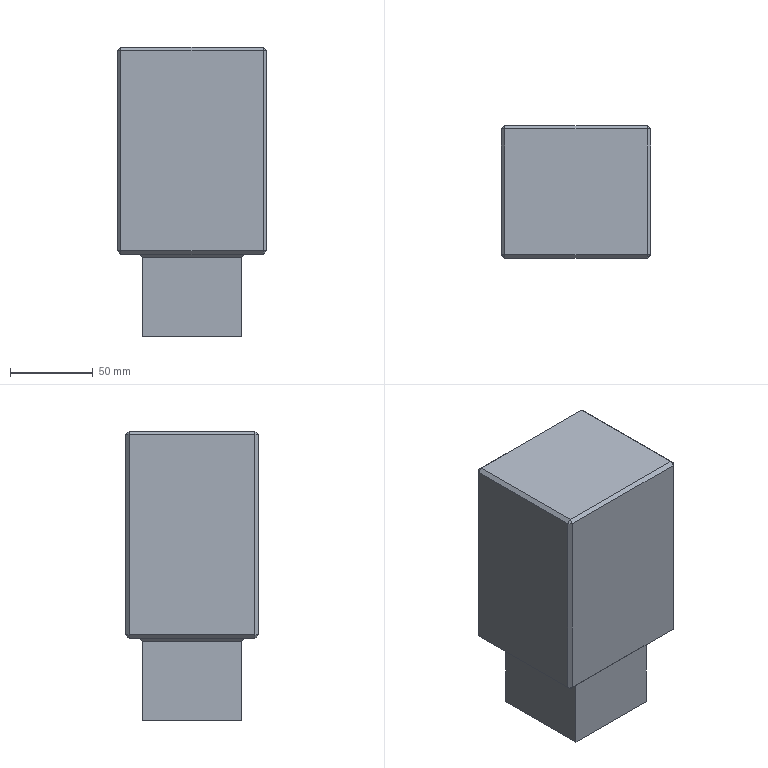Part | SolidWorks | features Boss 1, Chamfer 1, Cut 1, Extrusion 1 | 1 solid | 38 faces | box 90 x 80 x 175 mm | volume 1069126 mm3 | plane 36 | cylinder 2 | commonest cylinder face diameters 12 x2
STEP:
#1=CARTESIAN_POINT('',(36.,30.,80.));
#2=VERTEX_POINT('',#1);
#3=CARTESIAN_POINT('',(24.,30.,80.));
#4=VERTEX_POINT('',#3);
#5=CARTESIAN_POINT('',(30.,30.,80.));
#6=DIRECTION('',(0.,0.,-1.));
#7=DIRECTION('',(-1.,0.,0.));
#8=AXIS2_PLACEMENT_3D('',#5,#6,#7);
#9=CIRCLE('',#8,6.);
#10=EDGE_CURVE('',#2,#4,#9,.T.);
#11=ORIENTED_EDGE('',*,*,#10,.F.);
#12=CARTESIAN_POINT('',(36.,30.,0.));
#13=VERTEX_POINT('',#12);
#14=CARTESIAN_POINT('',(36.,30.,80.));
#15=DIRECTION('',(0.,0.,-1.));
#16=VECTOR('',#15,1000.);
#17=LINE('',#14,#16);
#18=EDGE_CURVE('',#2,#13,#17,.T.);
#19=ORIENTED_EDGE('',*,*,#18,.T.);
#20=CARTESIAN_POINT('',(24.,30.,0.));
#21=VERTEX_POINT('',#20);
#22=CARTESIAN_POINT('',(30.,30.,0.));
#23=DIRECTION('',(0.,0.,-1.));
#24=DIRECTION('',(-1.,0.,0.));
#25=AXIS2_PLACEMENT_3D('',#22,#23,#24);
#26=CIRCLE('',#25,6.);
#27=EDGE_CURVE('',#13,#21,#26,.T.);
#28=ORIENTED_EDGE('',*,*,#27,.T.);
#29=CARTESIAN_POINT('',(24.,30.,80.));
#30=DIRECTION('',(0.,0.,-1.));
#31=VECTOR('',#30,1000.);
#32=LINE('',#29,#31);
#33=EDGE_CURVE('',#4,#21,#32,.T.);
#34=ORIENTED_EDGE('',*,*,#33,.F.);
#35=EDGE_LOOP('',(#11,#19,#28,#34));
#36=FACE_OUTER_BOUND('',#35,.T.);
#37=CARTESIAN_POINT('',(30.,30.,80.));
#38=DIRECTION('',(0.,0.,-1.));
#39=DIRECTION('',(-1.,0.,0.));
#40=AXIS2_PLACEMENT_3D('',#37,#38,#39);
#41=CYLINDRICAL_SURFACE('',#40,6.);
#42=ADVANCED_FACE('',(#36),#41,.F.);
#43=CARTESIAN_POINT('',(0.,0.,48.));
#44=VERTEX_POINT('',#43);
#45=CARTESIAN_POINT('',(0.,0.,0.));
#46=VERTEX_POINT('',#45);
#47=CARTESIAN_POINT('',(0.,0.,50.));
#48=DIRECTION('',(0.,0.,-1.));
#49=VECTOR('',#48,1000.);
#50=LINE('',#47,#49);
#51=EDGE_CURVE('',#44,#46,#50,.T.);
#52=ORIENTED_EDGE('',*,*,#51,.F.);
#53=CARTESIAN_POINT('',(0.,60.,48.));
#54=VERTEX_POINT('',#53);
#55=CARTESIAN_POINT('',(0.,60.,48.));
#56=DIRECTION('',(0.,1.,0.));
#57=VECTOR('',#56,1000.);
#58=LINE('',#55,#57);
#59=EDGE_CURVE('',#44,#54,#58,.T.);
#60=ORIENTED_EDGE('',*,*,#59,.T.);
#61=CARTESIAN_POINT('',(0.,60.,0.));
#62=VERTEX_POINT('',#61);
#63=CARTESIAN_POINT('',(0.,60.,50.));
#64=DIRECTION('',(0.,0.,-1.));
#65=VECTOR('',#64,1000.);
#66=LINE('',#63,#65);
#67=EDGE_CURVE('',#54,#62,#66,.T.);
#68=ORIENTED_EDGE('',*,*,#67,.T.);
#69=CARTESIAN_POINT('',(0.,0.,0.));
#70=DIRECTION('',(0.,-1.,0.));
#71=VECTOR('',#70,1000.);
#72=LINE('',#69,#71);
#73=EDGE_CURVE('',#62,#46,#72,.T.);
#74=ORIENTED_EDGE('',*,*,#73,.T.);
#75=EDGE_LOOP('',(#52,#60,#68,#74));
#76=FACE_OUTER_BOUND('',#75,.T.);
#77=CARTESIAN_POINT('',(0.,0.,50.));
#78=DIRECTION('',(1.,0.,0.));
#79=DIRECTION('',(0.,0.,-1.));
#80=AXIS2_PLACEMENT_3D('',#77,#78,#79);
#81=PLANE('',#80);
#82=ADVANCED_FACE('',(#76),#81,.F.);
#83=CARTESIAN_POINT('',(60.,0.,48.));
#84=VERTEX_POINT('',#83);
#85=CARTESIAN_POINT('',(60.,0.,0.));
#86=VERTEX_POINT('',#85);
#87=CARTESIAN_POINT('',(60.,0.,50.));
#88=DIRECTION('',(0.,0.,-1.));
#89=VECTOR('',#88,1000.);
#90=LINE('',#87,#89);
#91=EDGE_CURVE('',#84,#86,#90,.T.);
#92=ORIENTED_EDGE('',*,*,#91,.F.);
#93=CARTESIAN_POINT('',(0.,0.,48.));
#94=DIRECTION('',(-1.,0.,0.));
#95=VECTOR('',#94,1000.);
#96=LINE('',#93,#95);
#97=EDGE_CURVE('',#84,#44,#96,.T.);
#98=ORIENTED_EDGE('',*,*,#97,.T.);
#99=ORIENTED_EDGE('',*,*,#51,.T.);
#100=CARTESIAN_POINT('',(0.,0.,0.));
#101=DIRECTION('',(1.,0.,0.));
#102=VECTOR('',#101,1000.);
#103=LINE('',#100,#102);
#104=EDGE_CURVE('',#46,#86,#103,.T.);
#105=ORIENTED_EDGE('',*,*,#104,.T.);
#106=EDGE_LOOP('',(#92,#98,#99,#105));
#107=FACE_OUTER_BOUND('',#106,.T.);
#108=CARTESIAN_POINT('',(0.,0.,50.));
#109=DIRECTION('',(0.,1.,0.));
#110=DIRECTION('',(0.,0.,1.));
#111=AXIS2_PLACEMENT_3D('',#108,#109,#110);
#112=PLANE('',#111);
#113=ADVANCED_FACE('',(#107),#112,.F.);
#114=CARTESIAN_POINT('',(60.,60.,48.));
#115=VERTEX_POINT('',#114);
#116=CARTESIAN_POINT('',(60.,60.,0.));
#117=VERTEX_POINT('',#116);
#118=CARTESIAN_POINT('',(60.,60.,50.));
#119=DIRECTION('',(0.,0.,-1.));
#120=VECTOR('',#119,1000.);
#121=LINE('',#118,#120);
#122=EDGE_CURVE('',#115,#117,#121,.T.);
#123=ORIENTED_EDGE('',*,*,#122,.F.);
#124=CARTESIAN_POINT('',(60.,0.,48.));
#125=DIRECTION('',(0.,-1.,0.));
#126=VECTOR('',#125,1000.);
#127=LINE('',#124,#126);
#128=EDGE_CURVE('',#115,#84,#127,.T.);
#129=ORIENTED_EDGE('',*,*,#128,.T.);
#130=ORIENTED_EDGE('',*,*,#91,.T.);
#131=CARTESIAN_POINT('',(60.,0.,0.));
#132=DIRECTION('',(0.,1.,0.));
#133=VECTOR('',#132,1000.);
#134=LINE('',#131,#133);
#135=EDGE_CURVE('',#86,#117,#134,.T.);
#136=ORIENTED_EDGE('',*,*,#135,.T.);
#137=EDGE_LOOP('',(#123,#129,#130,#136));
#138=FACE_OUTER_BOUND('',#137,.T.);
#139=CARTESIAN_POINT('',(60.,0.,50.));
#140=DIRECTION('',(-1.,0.,0.));
#141=DIRECTION('',(0.,0.,1.));
#142=AXIS2_PLACEMENT_3D('',#139,#140,#141);
#143=PLANE('',#142);
#144=ADVANCED_FACE('',(#138),#143,.F.);
#145=ORIENTED_EDGE('',*,*,#67,.F.);
#146=CARTESIAN_POINT('',(60.,60.,48.));
#147=DIRECTION('',(1.,0.,0.));
#148=VECTOR('',#147,1000.);
#149=LINE('',#146,#148);
#150=EDGE_CURVE('',#54,#115,#149,.T.);
#151=ORIENTED_EDGE('',*,*,#150,.T.);
#152=ORIENTED_EDGE('',*,*,#122,.T.);
#153=CARTESIAN_POINT('',(0.,60.,0.));
#154=DIRECTION('',(-1.,0.,0.));
#155=VECTOR('',#154,1000.);
#156=LINE('',#153,#155);
#157=EDGE_CURVE('',#117,#62,#156,.T.);
#158=ORIENTED_EDGE('',*,*,#157,.T.);
#159=EDGE_LOOP('',(#145,#151,#152,#158));
#160=FACE_OUTER_BOUND('',#159,.T.);
#161=CARTESIAN_POINT('',(0.,60.,50.));
#162=DIRECTION('',(0.,-1.,0.));
#163=DIRECTION('',(0.,0.,-1.));
#164=AXIS2_PLACEMENT_3D('',#161,#162,#163);
#165=PLANE('',#164);
#166=ADVANCED_FACE('',(#160),#165,.F.);
#167=CARTESIAN_POINT('',(30.,30.,0.));
#168=DIRECTION('',(0.,0.,-1.));
#169=DIRECTION('',(-1.,0.,0.));
#170=AXIS2_PLACEMENT_3D('',#167,#168,#169);
#171=CIRCLE('',#170,6.);
#172=EDGE_CURVE('',#21,#13,#171,.T.);
#173=ORIENTED_EDGE('',*,*,#172,.F.);
#174=ORIENTED_EDGE('',*,*,#27,.F.);
#175=EDGE_LOOP('',(#173,#174));
#176=FACE_BOUND('',#175,.T.);
#177=ORIENTED_EDGE('',*,*,#73,.F.);
#178=ORIENTED_EDGE('',*,*,#157,.F.);
#179=ORIENTED_EDGE('',*,*,#135,.F.);
#180=ORIENTED_EDGE('',*,*,#104,.F.);
#181=EDGE_LOOP('',(#177,#178,#179,#180));
#182=FACE_OUTER_BOUND('',#181,.T.);
#183=CARTESIAN_POINT('',(0.,60.,0.));
#184=DIRECTION('',(0.,0.,-1.));
#185=DIRECTION('',(-1.,0.,0.));
#186=AXIS2_PLACEMENT_3D('',#183,#184,#185);
#187=PLANE('',#186);
#188=ADVANCED_FACE('',(#176,#182),#187,.T.);
#189=CARTESIAN_POINT('',(-2.,-2.,50.));
#190=VERTEX_POINT('',#189);
#191=CARTESIAN_POINT('',(62.,-2.,50.));
#192=VERTEX_POINT('',#191);
#193=CARTESIAN_POINT('',(60.,-2.,50.));
#194=DIRECTION('',(1.,0.,0.));
#195=VECTOR('',#194,1000.);
#196=LINE('',#193,#195);
#197=EDGE_CURVE('',#190,#192,#196,.T.);
#198=ORIENTED_EDGE('',*,*,#197,.T.);
#199=CARTESIAN_POINT('',(62.,62.,50.));
#200=VERTEX_POINT('',#199);
#201=CARTESIAN_POINT('',(62.,60.,50.));
#202=DIRECTION('',(0.,1.,0.));
#203=VECTOR('',#202,1000.);
#204=LINE('',#201,#203);
#205=EDGE_CURVE('',#192,#200,#204,.T.);
#206=ORIENTED_EDGE('',*,*,#205,.T.);
#207=CARTESIAN_POINT('',(-2.,62.,50.));
#208=VERTEX_POINT('',#207);
#209=CARTESIAN_POINT('',(0.,62.,50.));
#210=DIRECTION('',(-1.,0.,0.));
#211=VECTOR('',#210,1000.);
#212=LINE('',#209,#211);
#213=EDGE_CURVE('',#200,#208,#212,.T.);
#214=ORIENTED_EDGE('',*,*,#213,.T.);
#215=CARTESIAN_POINT('',(-2.,0.,50.));
#216=DIRECTION('',(0.,-1.,0.));
#217=VECTOR('',#216,1000.);
#218=LINE('',#215,#217);
#219=EDGE_CURVE('',#208,#190,#218,.T.);
#220=ORIENTED_EDGE('',*,*,#219,.T.);
#221=EDGE_LOOP('',(#198,#206,#214,#220));
#222=FACE_BOUND('',#221,.T.);
#223=CARTESIAN_POINT('',(73.,68.,50.));
#224=VERTEX_POINT('',#223);
#225=CARTESIAN_POINT('',(73.,-8.,50.));
#226=VERTEX_POINT('',#225);
#227=CARTESIAN_POINT('',(73.,-10.,50.));
#228=DIRECTION('',(0.,-1.,0.));
#229=VECTOR('',#228,1000.);
#230=LINE('',#227,#229);
#231=EDGE_CURVE('',#224,#226,#230,.T.);
#232=ORIENTED_EDGE('',*,*,#231,.T.);
#233=CARTESIAN_POINT('',(-13.,-8.,50.));
#234=VERTEX_POINT('',#233);
#235=CARTESIAN_POINT('',(-15.,-8.,50.));
#236=DIRECTION('',(-1.,0.,0.));
#237=VECTOR('',#236,1000.);
#238=LINE('',#235,#237);
#239=EDGE_CURVE('',#226,#234,#238,.T.);
#240=ORIENTED_EDGE('',*,*,#239,.T.);
#241=CARTESIAN_POINT('',(-13.,68.,50.));
#242=VERTEX_POINT('',#241);
#243=CARTESIAN_POINT('',(-13.,-10.,50.));
#244=DIRECTION('',(0.,1.,0.));
#245=VECTOR('',#244,1000.);
#246=LINE('',#243,#245);
#247=EDGE_CURVE('',#234,#242,#246,.T.);
#248=ORIENTED_EDGE('',*,*,#247,.T.);
#249=CARTESIAN_POINT('',(-15.,68.,50.));
#250=DIRECTION('',(1.,0.,0.));
#251=VECTOR('',#250,1000.);
#252=LINE('',#249,#251);
#253=EDGE_CURVE('',#242,#224,#252,.T.);
#254=ORIENTED_EDGE('',*,*,#253,.T.);
#255=EDGE_LOOP('',(#232,#240,#248,#254));
#256=FACE_OUTER_BOUND('',#255,.T.);
#257=CARTESIAN_POINT('',(-15.,-10.,50.));
#258=DIRECTION('',(0.,0.,1.));
#259=DIRECTION('',(1.,0.,0.));
#260=AXIS2_PLACEMENT_3D('',#257,#258,#259);
#261=PLANE('',#260);
#262=ADVANCED_FACE('',(#222,#256),#261,.F.);
#263=CARTESIAN_POINT('',(-15.,-8.,173.));
#264=VERTEX_POINT('',#263);
#265=CARTESIAN_POINT('',(-15.,68.,173.));
#266=VERTEX_POINT('',#265);
#267=CARTESIAN_POINT('',(-15.,70.,173.));
#268=DIRECTION('',(0.,1.,0.));
#269=VECTOR('',#268,1000.);
#270=LINE('',#267,#269);
#271=EDGE_CURVE('',#264,#266,#270,.T.);
#272=ORIENTED_EDGE('',*,*,#271,.T.);
#273=CARTESIAN_POINT('',(-15.,68.,52.));
#274=VERTEX_POINT('',#273);
#275=CARTESIAN_POINT('',(-15.,68.,175.));
#276=DIRECTION('',(0.,0.,-1.));
#277=VECTOR('',#276,1000.);
#278=LINE('',#275,#277);
#279=EDGE_CURVE('',#266,#274,#278,.T.);
#280=ORIENTED_EDGE('',*,*,#279,.T.);
#281=CARTESIAN_POINT('',(-15.,-8.,52.));
#282=VERTEX_POINT('',#281);
#283=CARTESIAN_POINT('',(-15.,70.,52.));
#284=DIRECTION('',(0.,-1.,0.));
#285=VECTOR('',#284,1000.);
#286=LINE('',#283,#285);
#287=EDGE_CURVE('',#274,#282,#286,.T.);
#288=ORIENTED_EDGE('',*,*,#287,.T.);
#289=CARTESIAN_POINT('',(-15.,-8.,175.));
#290=DIRECTION('',(0.,0.,1.));
#291=VECTOR('',#290,1000.);
#292=LINE('',#289,#291);
#293=EDGE_CURVE('',#282,#264,#292,.T.);
#294=ORIENTED_EDGE('',*,*,#293,.T.);
#295=EDGE_LOOP('',(#272,#280,#288,#294));
#296=FACE_OUTER_BOUND('',#295,.T.);
#297=CARTESIAN_POINT('',(-15.,70.,175.));
#298=DIRECTION('',(1.,0.,0.));
#299=DIRECTION('',(0.,1.,0.));
#300=AXIS2_PLACEMENT_3D('',#297,#298,#299);
#301=PLANE('',#300);
#302=ADVANCED_FACE('',(#296),#301,.F.);
#303=CARTESIAN_POINT('',(73.,-10.,52.));
#304=VERTEX_POINT('',#303);
#305=CARTESIAN_POINT('',(73.,-10.,173.));
#306=VERTEX_POINT('',#305);
#307=CARTESIAN_POINT('',(73.,-10.,175.));
#308=DIRECTION('',(0.,0.,1.));
#309=VECTOR('',#308,1000.);
#310=LINE('',#307,#309);
#311=EDGE_CURVE('',#304,#306,#310,.T.);
#312=ORIENTED_EDGE('',*,*,#311,.T.);
#313=CARTESIAN_POINT('',(-13.,-10.,173.));
#314=VERTEX_POINT('',#313);
#315=CARTESIAN_POINT('',(-15.,-10.,173.));
#316=DIRECTION('',(-1.,0.,0.));
#317=VECTOR('',#316,1000.);
#318=LINE('',#315,#317);
#319=EDGE_CURVE('',#306,#314,#318,.T.);
#320=ORIENTED_EDGE('',*,*,#319,.T.);
#321=CARTESIAN_POINT('',(-13.,-10.,52.));
#322=VERTEX_POINT('',#321);
#323=CARTESIAN_POINT('',(-13.,-10.,175.));
#324=DIRECTION('',(0.,0.,-1.));
#325=VECTOR('',#324,1000.);
#326=LINE('',#323,#325);
#327=EDGE_CURVE('',#314,#322,#326,.T.);
#328=ORIENTED_EDGE('',*,*,#327,.T.);
#329=CARTESIAN_POINT('',(-15.,-10.,52.));
#330=DIRECTION('',(1.,0.,0.));
#331=VECTOR('',#330,1000.);
#332=LINE('',#329,#331);
#333=EDGE_CURVE('',#322,#304,#332,.T.);
#334=ORIENTED_EDGE('',*,*,#333,.T.);
#335=EDGE_LOOP('',(#312,#320,#328,#334));
#336=FACE_OUTER_BOUND('',#335,.T.);
#337=CARTESIAN_POINT('',(-15.,-10.,175.));
#338=DIRECTION('',(0.,1.,0.));
#339=DIRECTION('',(-1.,0.,0.));
#340=AXIS2_PLACEMENT_3D('',#337,#338,#339);
#341=PLANE('',#340);
#342=ADVANCED_FACE('',(#336),#341,.F.);
#343=CARTESIAN_POINT('',(75.,-8.,52.));
#344=VERTEX_POINT('',#343);
#345=CARTESIAN_POINT('',(75.,68.,52.));
#346=VERTEX_POINT('',#345);
#347=CARTESIAN_POINT('',(75.,70.,52.));
#348=DIRECTION('',(0.,1.,0.));
#349=VECTOR('',#348,1000.);
#350=LINE('',#347,#349);
#351=EDGE_CURVE('',#344,#346,#350,.T.);
#352=ORIENTED_EDGE('',*,*,#351,.T.);
#353=CARTESIAN_POINT('',(75.,68.,173.));
#354=VERTEX_POINT('',#353);
#355=CARTESIAN_POINT('',(75.,68.,175.));
#356=DIRECTION('',(0.,0.,1.));
#357=VECTOR('',#356,1000.);
#358=LINE('',#355,#357);
#359=EDGE_CURVE('',#346,#354,#358,.T.);
#360=ORIENTED_EDGE('',*,*,#359,.T.);
#361=CARTESIAN_POINT('',(75.,-8.,173.));
#362=VERTEX_POINT('',#361);
#363=CARTESIAN_POINT('',(75.,-10.,173.));
#364=DIRECTION('',(0.,-1.,0.));
#365=VECTOR('',#364,1000.);
#366=LINE('',#363,#365);
#367=EDGE_CURVE('',#354,#362,#366,.T.);
#368=ORIENTED_EDGE('',*,*,#367,.T.);
#369=CARTESIAN_POINT('',(75.,-8.,175.));
#370=DIRECTION('',(0.,0.,-1.));
#371=VECTOR('',#370,1000.);
#372=LINE('',#369,#371);
#373=EDGE_CURVE('',#362,#344,#372,.T.);
#374=ORIENTED_EDGE('',*,*,#373,.T.);
#375=EDGE_LOOP('',(#352,#360,#368,#374));
#376=FACE_OUTER_BOUND('',#375,.T.);
#377=CARTESIAN_POINT('',(75.,70.,175.));
#378=DIRECTION('',(-1.,0.,0.));
#379=DIRECTION('',(0.,-1.,0.));
#380=AXIS2_PLACEMENT_3D('',#377,#378,#379);
#381=PLANE('',#380);
#382=ADVANCED_FACE('',(#376),#381,.F.);
#383=CARTESIAN_POINT('',(-13.,70.,173.));
#384=VERTEX_POINT('',#383);
#385=CARTESIAN_POINT('',(73.,70.,173.));
#386=VERTEX_POINT('',#385);
#387=CARTESIAN_POINT('',(75.,70.,173.));
#388=DIRECTION('',(1.,0.,0.));
#389=VECTOR('',#388,1000.);
#390=LINE('',#387,#389);
#391=EDGE_CURVE('',#384,#386,#390,.T.);
#392=ORIENTED_EDGE('',*,*,#391,.T.);
#393=CARTESIAN_POINT('',(73.,70.,52.));
#394=VERTEX_POINT('',#393);
#395=CARTESIAN_POINT('',(73.,70.,175.));
#396=DIRECTION('',(0.,0.,-1.));
#397=VECTOR('',#396,1000.);
#398=LINE('',#395,#397);
#399=EDGE_CURVE('',#386,#394,#398,.T.);
#400=ORIENTED_EDGE('',*,*,#399,.T.);
#401=CARTESIAN_POINT('',(-13.,70.,52.));
#402=VERTEX_POINT('',#401);
#403=CARTESIAN_POINT('',(-15.,70.,52.));
#404=DIRECTION('',(-1.,0.,0.));
#405=VECTOR('',#404,1000.);
#406=LINE('',#403,#405);
#407=EDGE_CURVE('',#394,#402,#406,.T.);
#408=ORIENTED_EDGE('',*,*,#407,.T.);
#409=CARTESIAN_POINT('',(-13.,70.,175.));
#410=DIRECTION('',(0.,0.,1.));
#411=VECTOR('',#410,1000.);
#412=LINE('',#409,#411);
#413=EDGE_CURVE('',#402,#384,#412,.T.);
#414=ORIENTED_EDGE('',*,*,#413,.T.);
#415=EDGE_LOOP('',(#392,#400,#408,#414));
#416=FACE_OUTER_BOUND('',#415,.T.);
#417=CARTESIAN_POINT('',(-15.,70.,175.));
#418=DIRECTION('',(0.,-1.,0.));
#419=DIRECTION('',(0.,0.,-1.));
#420=AXIS2_PLACEMENT_3D('',#417,#418,#419);
#421=PLANE('',#420);
#422=ADVANCED_FACE('',(#416),#421,.F.);
#423=CARTESIAN_POINT('',(73.,-8.,175.));
#424=VERTEX_POINT('',#423);
#425=CARTESIAN_POINT('',(73.,68.,175.));
#426=VERTEX_POINT('',#425);
#427=CARTESIAN_POINT('',(73.,70.,175.));
#428=DIRECTION('',(0.,1.,0.));
#429=VECTOR('',#428,1000.);
#430=LINE('',#427,#429);
#431=EDGE_CURVE('',#424,#426,#430,.T.);
#432=ORIENTED_EDGE('',*,*,#431,.T.);
#433=CARTESIAN_POINT('',(-13.,68.,175.));
#434=VERTEX_POINT('',#433);
#435=CARTESIAN_POINT('',(-15.,68.,175.));
#436=DIRECTION('',(-1.,0.,0.));
#437=VECTOR('',#436,1000.);
#438=LINE('',#435,#437);
#439=EDGE_CURVE('',#426,#434,#438,.T.);
#440=ORIENTED_EDGE('',*,*,#439,.T.);
#441=CARTESIAN_POINT('',(-13.,-8.,175.));
#442=VERTEX_POINT('',#441);
#443=CARTESIAN_POINT('',(-13.,-10.,175.));
#444=DIRECTION('',(0.,-1.,0.));
#445=VECTOR('',#444,1000.);
#446=LINE('',#443,#445);
#447=EDGE_CURVE('',#434,#442,#446,.T.);
#448=ORIENTED_EDGE('',*,*,#447,.T.);
#449=CARTESIAN_POINT('',(75.,-8.,175.));
#450=DIRECTION('',(1.,0.,0.));
#451=VECTOR('',#450,1000.);
#452=LINE('',#449,#451);
#453=EDGE_CURVE('',#442,#424,#452,.T.);
#454=ORIENTED_EDGE('',*,*,#453,.T.);
#455=EDGE_LOOP('',(#432,#440,#448,#454));
#456=FACE_OUTER_BOUND('',#455,.T.);
#457=CARTESIAN_POINT('',(-15.,-10.,175.));
#458=DIRECTION('',(0.,0.,1.));
#459=DIRECTION('',(1.,0.,0.));
#460=AXIS2_PLACEMENT_3D('',#457,#458,#459);
#461=PLANE('',#460);
#462=ADVANCED_FACE('',(#456),#461,.T.);
#463=CARTESIAN_POINT('',(-6.333,66.333,54.333));
#464=DIRECTION('',(-0.5774,0.5774,0.5774));
#465=VECTOR('',#464,1000.);
#466=LINE('',#463,#465);
#467=EDGE_CURVE('',#54,#208,#466,.T.);
#468=ORIENTED_EDGE('',*,*,#467,.F.);
#469=ORIENTED_EDGE('',*,*,#59,.F.);
#470=CARTESIAN_POINT('',(-4.667,-4.667,52.667));
#471=DIRECTION('',(0.5774,0.5774,-0.5774));
#472=VECTOR('',#471,1000.);
#473=LINE('',#470,#472);
#474=EDGE_CURVE('',#190,#44,#473,.T.);
#475=ORIENTED_EDGE('',*,*,#474,.F.);
#476=ORIENTED_EDGE('',*,*,#219,.F.);
#477=EDGE_LOOP('',(#468,#469,#475,#476));
#478=FACE_OUTER_BOUND('',#477,.T.);
#479=CARTESIAN_POINT('',(-2.,-10.,50.));
#480=DIRECTION('',(-0.7071,0.,-0.7071));
#481=DIRECTION('',(-0.7071,0.,0.7071));
#482=AXIS2_PLACEMENT_3D('',#479,#480,#481);
#483=PLANE('',#482);
#484=ADVANCED_FACE('',(#478),#483,.T.);
#485=ORIENTED_EDGE('',*,*,#474,.T.);
#486=ORIENTED_EDGE('',*,*,#97,.F.);
#487=CARTESIAN_POINT('',(36.333,23.667,24.333));
#488=DIRECTION('',(-0.5774,0.5774,-0.5774));
#489=VECTOR('',#488,1000.);
#490=LINE('',#487,#489);
#491=EDGE_CURVE('',#192,#84,#490,.T.);
#492=ORIENTED_EDGE('',*,*,#491,.F.);
#493=ORIENTED_EDGE('',*,*,#197,.F.);
#494=EDGE_LOOP('',(#485,#486,#492,#493));
#495=FACE_OUTER_BOUND('',#494,.T.);
#496=CARTESIAN_POINT('',(-15.,-2.,50.));
#497=DIRECTION('',(0.,-0.7071,-0.7071));
#498=DIRECTION('',(0.,0.7071,-0.7071));
#499=AXIS2_PLACEMENT_3D('',#496,#497,#498);
#500=PLANE('',#499);
#501=ADVANCED_FACE('',(#495),#500,.T.);
#502=ORIENTED_EDGE('',*,*,#467,.T.);
#503=ORIENTED_EDGE('',*,*,#213,.F.);
#504=CARTESIAN_POINT('',(36.333,36.333,24.333));
#505=DIRECTION('',(0.5774,0.5774,0.5774));
#506=VECTOR('',#505,1000.);
#507=LINE('',#504,#506);
#508=EDGE_CURVE('',#115,#200,#507,.T.);
#509=ORIENTED_EDGE('',*,*,#508,.F.);
#510=ORIENTED_EDGE('',*,*,#150,.F.);
#511=EDGE_LOOP('',(#502,#503,#509,#510));
#512=FACE_OUTER_BOUND('',#511,.T.);
#513=CARTESIAN_POINT('',(-15.,62.,50.));
#514=DIRECTION('',(0.,0.7071,-0.7071));
#515=DIRECTION('',(0.,0.7071,0.7071));
#516=AXIS2_PLACEMENT_3D('',#513,#514,#515);
#517=PLANE('',#516);
#518=ADVANCED_FACE('',(#512),#517,.T.);
#519=ORIENTED_EDGE('',*,*,#491,.T.);
#520=ORIENTED_EDGE('',*,*,#128,.F.);
#521=ORIENTED_EDGE('',*,*,#508,.T.);
#522=ORIENTED_EDGE('',*,*,#205,.F.);
#523=EDGE_LOOP('',(#519,#520,#521,#522));
#524=FACE_OUTER_BOUND('',#523,.T.);
#525=CARTESIAN_POINT('',(62.,-10.,50.));
#526=DIRECTION('',(0.7071,0.,-0.7071));
#527=DIRECTION('',(-0.7071,0.,-0.7071));
#528=AXIS2_PLACEMENT_3D('',#525,#526,#527);
#529=PLANE('',#528);
#530=ADVANCED_FACE('',(#524),#529,.T.);
#531=CARTESIAN_POINT('',(-13.,-10.,173.));
#532=DIRECTION('',(0.7071,-0.7071,0.));
#533=VECTOR('',#532,1000.);
#534=LINE('',#531,#533);
#535=EDGE_CURVE('',#264,#314,#534,.T.);
#536=ORIENTED_EDGE('',*,*,#535,.F.);
#537=ORIENTED_EDGE('',*,*,#293,.F.);
#538=CARTESIAN_POINT('',(-14.,-9.,52.));
#539=DIRECTION('',(-0.7071,0.7071,0.));
#540=VECTOR('',#539,1000.);
#541=LINE('',#538,#540);
#542=EDGE_CURVE('',#322,#282,#541,.T.);
#543=ORIENTED_EDGE('',*,*,#542,.F.);
#544=ORIENTED_EDGE('',*,*,#327,.F.);
#545=EDGE_LOOP('',(#536,#537,#543,#544));
#546=FACE_OUTER_BOUND('',#545,.T.);
#547=CARTESIAN_POINT('',(-13.,-10.,175.));
#548=DIRECTION('',(0.7071,0.7071,0.));
#549=DIRECTION('',(-0.7071,0.7071,0.));
#550=AXIS2_PLACEMENT_3D('',#547,#548,#549);
#551=PLANE('',#550);
#552=ADVANCED_FACE('',(#546),#551,.F.);
#553=CARTESIAN_POINT('',(-14.,-8.,174.));
#554=DIRECTION('',(0.7071,0.,0.7071));
#555=VECTOR('',#554,1000.);
#556=LINE('',#553,#555);
#557=EDGE_CURVE('',#264,#442,#556,.T.);
#558=ORIENTED_EDGE('',*,*,#557,.F.);
#559=ORIENTED_EDGE('',*,*,#535,.T.);
#560=CARTESIAN_POINT('',(-13.,-10.,173.));
#561=DIRECTION('',(0.,-0.7071,-0.7071));
#562=VECTOR('',#561,1000.);
#563=LINE('',#560,#562);
#564=EDGE_CURVE('',#442,#314,#563,.T.);
#565=ORIENTED_EDGE('',*,*,#564,.F.);
#566=EDGE_LOOP('',(#558,#559,#565));
#567=FACE_OUTER_BOUND('',#566,.T.);
#568=CARTESIAN_POINT('',(-13.,-10.,173.));
#569=DIRECTION('',(-0.5774,-0.5774,0.5774));
#570=DIRECTION('',(0.7071,-0.7071,0.));
#571=AXIS2_PLACEMENT_3D('',#568,#569,#570);
#572=PLANE('',#571);
#573=ADVANCED_FACE('',(#567),#572,.T.);
#574=CARTESIAN_POINT('',(-13.,-8.,50.));
#575=DIRECTION('',(0.,0.7071,-0.7071));
#576=VECTOR('',#575,1000.);
#577=LINE('',#574,#576);
#578=EDGE_CURVE('',#322,#234,#577,.T.);
#579=ORIENTED_EDGE('',*,*,#578,.F.);
#580=ORIENTED_EDGE('',*,*,#542,.T.);
#581=CARTESIAN_POINT('',(-13.,-8.,50.));
#582=DIRECTION('',(-0.7071,0.,0.7071));
#583=VECTOR('',#582,1000.);
#584=LINE('',#581,#583);
#585=EDGE_CURVE('',#234,#282,#584,.T.);
#586=ORIENTED_EDGE('',*,*,#585,.F.);
#587=EDGE_LOOP('',(#579,#580,#586));
#588=FACE_OUTER_BOUND('',#587,.T.);
#589=CARTESIAN_POINT('',(-13.,-8.,50.));
#590=DIRECTION('',(-0.5774,-0.5774,-0.5774));
#591=DIRECTION('',(-0.7071,0.,0.7071));
#592=AXIS2_PLACEMENT_3D('',#589,#590,#591);
#593=PLANE('',#592);
#594=ADVANCED_FACE('',(#588),#593,.T.);
#595=ORIENTED_EDGE('',*,*,#564,.T.);
#596=ORIENTED_EDGE('',*,*,#319,.F.);
#597=CARTESIAN_POINT('',(73.,-9.,174.));
#598=DIRECTION('',(0.,-0.7071,-0.7071));
#599=VECTOR('',#598,1000.);
#600=LINE('',#597,#599);
#601=EDGE_CURVE('',#424,#306,#600,.T.);
#602=ORIENTED_EDGE('',*,*,#601,.F.);
#603=ORIENTED_EDGE('',*,*,#453,.F.);
#604=EDGE_LOOP('',(#595,#596,#602,#603));
#605=FACE_OUTER_BOUND('',#604,.T.);
#606=CARTESIAN_POINT('',(-15.,-8.,175.));
#607=DIRECTION('',(0.,-0.7071,0.7071));
#608=DIRECTION('',(0.,-0.7071,-0.7071));
#609=AXIS2_PLACEMENT_3D('',#606,#607,#608);
#610=PLANE('',#609);
#611=ADVANCED_FACE('',(#605),#610,.T.);
#612=ORIENTED_EDGE('',*,*,#557,.T.);
#613=ORIENTED_EDGE('',*,*,#447,.F.);
#614=CARTESIAN_POINT('',(-13.,68.,175.));
#615=DIRECTION('',(0.7071,0.,0.7071));
#616=VECTOR('',#615,1000.);
#617=LINE('',#614,#616);
#618=EDGE_CURVE('',#266,#434,#617,.T.);
#619=ORIENTED_EDGE('',*,*,#618,.F.);
#620=ORIENTED_EDGE('',*,*,#271,.F.);
#621=EDGE_LOOP('',(#612,#613,#619,#620));
#622=FACE_OUTER_BOUND('',#621,.T.);
#623=CARTESIAN_POINT('',(-13.,-10.,175.));
#624=DIRECTION('',(-0.7071,0.,0.7071));
#625=DIRECTION('',(0.7071,0.,0.7071));
#626=AXIS2_PLACEMENT_3D('',#623,#624,#625);
#627=PLANE('',#626);
#628=ADVANCED_FACE('',(#622),#627,.T.);
#629=CARTESIAN_POINT('',(-13.,70.,52.));
#630=DIRECTION('',(0.7071,0.7071,0.));
#631=VECTOR('',#630,1000.);
#632=LINE('',#629,#631);
#633=EDGE_CURVE('',#274,#402,#632,.T.);
#634=ORIENTED_EDGE('',*,*,#633,.F.);
#635=ORIENTED_EDGE('',*,*,#279,.F.);
#636=CARTESIAN_POINT('',(-14.,69.,173.));
#637=DIRECTION('',(-0.7071,-0.7071,0.));
#638=VECTOR('',#637,1000.);
#639=LINE('',#636,#638);
#640=EDGE_CURVE('',#384,#266,#639,.T.);
#641=ORIENTED_EDGE('',*,*,#640,.F.);
#642=ORIENTED_EDGE('',*,*,#413,.F.);
#643=EDGE_LOOP('',(#634,#635,#641,#642));
#644=FACE_OUTER_BOUND('',#643,.T.);
#645=CARTESIAN_POINT('',(-15.,68.,175.));
#646=DIRECTION('',(0.7071,-0.7071,0.));
#647=DIRECTION('',(0.7071,0.7071,0.));
#648=AXIS2_PLACEMENT_3D('',#645,#646,#647);
#649=PLANE('',#648);
#650=ADVANCED_FACE('',(#644),#649,.F.);
#651=ORIENTED_EDGE('',*,*,#585,.T.);
#652=ORIENTED_EDGE('',*,*,#287,.F.);
#653=CARTESIAN_POINT('',(-14.,68.,51.));
#654=DIRECTION('',(-0.7071,0.,0.7071));
#655=VECTOR('',#654,1000.);
#656=LINE('',#653,#655);
#657=EDGE_CURVE('',#242,#274,#656,.T.);
#658=ORIENTED_EDGE('',*,*,#657,.F.);
#659=ORIENTED_EDGE('',*,*,#247,.F.);
#660=EDGE_LOOP('',(#651,#652,#658,#659));
#661=FACE_OUTER_BOUND('',#660,.T.);
#662=CARTESIAN_POINT('',(-15.,70.,52.));
#663=DIRECTION('',(0.7071,0.,0.7071));
#664=DIRECTION('',(0.7071,0.,-0.7071));
#665=AXIS2_PLACEMENT_3D('',#662,#663,#664);
#666=PLANE('',#665);
#667=ADVANCED_FACE('',(#661),#666,.F.);
#668=ORIENTED_EDGE('',*,*,#578,.T.);
#669=ORIENTED_EDGE('',*,*,#239,.F.);
#670=CARTESIAN_POINT('',(73.,-9.,51.));
#671=DIRECTION('',(0.,0.7071,-0.7071));
#672=VECTOR('',#671,1000.);
#673=LINE('',#670,#672);
#674=EDGE_CURVE('',#304,#226,#673,.T.);
#675=ORIENTED_EDGE('',*,*,#674,.F.);
#676=ORIENTED_EDGE('',*,*,#333,.F.);
#677=EDGE_LOOP('',(#668,#669,#675,#676));
#678=FACE_OUTER_BOUND('',#677,.T.);
#679=CARTESIAN_POINT('',(-15.,-10.,52.));
#680=DIRECTION('',(0.,0.7071,0.7071));
#681=DIRECTION('',(0.,-0.7071,0.7071));
#682=AXIS2_PLACEMENT_3D('',#679,#680,#681);
#683=PLANE('',#682);
#684=ADVANCED_FACE('',(#678),#683,.F.);
#685=CARTESIAN_POINT('',(75.,-8.,173.));
#686=DIRECTION('',(0.7071,0.7071,0.));
#687=VECTOR('',#686,1000.);
#688=LINE('',#685,#687);
#689=EDGE_CURVE('',#306,#362,#688,.T.);
#690=ORIENTED_EDGE('',*,*,#689,.F.);
#691=ORIENTED_EDGE('',*,*,#311,.F.);
#692=CARTESIAN_POINT('',(75.,-8.,52.));
#693=DIRECTION('',(-0.7071,-0.7071,0.));
#694=VECTOR('',#693,1000.);
#695=LINE('',#692,#694);
#696=EDGE_CURVE('',#344,#304,#695,.T.);
#697=ORIENTED_EDGE('',*,*,#696,.F.);
#698=ORIENTED_EDGE('',*,*,#373,.F.);
#699=EDGE_LOOP('',(#690,#691,#697,#698));
#700=FACE_OUTER_BOUND('',#699,.T.);
#701=CARTESIAN_POINT('',(75.,-8.,175.));
#702=DIRECTION('',(-0.7071,0.7071,0.));
#703=DIRECTION('',(-0.7071,-0.7071,0.));
#704=AXIS2_PLACEMENT_3D('',#701,#702,#703);
#705=PLANE('',#704);
#706=ADVANCED_FACE('',(#700),#705,.F.);
#707=ORIENTED_EDGE('',*,*,#601,.T.);
#708=ORIENTED_EDGE('',*,*,#689,.T.);
#709=CARTESIAN_POINT('',(75.,-8.,173.));
#710=DIRECTION('',(0.7071,0.,-0.7071));
#711=VECTOR('',#710,1000.);
#712=LINE('',#709,#711);
#713=EDGE_CURVE('',#424,#362,#712,.T.);
#714=ORIENTED_EDGE('',*,*,#713,.F.);
#715=EDGE_LOOP('',(#707,#708,#714));
#716=FACE_OUTER_BOUND('',#715,.T.);
#717=CARTESIAN_POINT('',(75.,-8.,173.));
#718=DIRECTION('',(0.5774,-0.5774,0.5774));
#719=DIRECTION('',(0.7071,0.7071,0.));
#720=AXIS2_PLACEMENT_3D('',#717,#718,#719);
#721=PLANE('',#720);
#722=ADVANCED_FACE('',(#716),#721,.T.);
#723=ORIENTED_EDGE('',*,*,#640,.T.);
#724=ORIENTED_EDGE('',*,*,#618,.T.);
#725=CARTESIAN_POINT('',(-13.,68.,175.));
#726=DIRECTION('',(0.,-0.7071,0.7071));
#727=VECTOR('',#726,1000.);
#728=LINE('',#725,#727);
#729=EDGE_CURVE('',#384,#434,#728,.T.);
#730=ORIENTED_EDGE('',*,*,#729,.F.);
#731=EDGE_LOOP('',(#723,#724,#730));
#732=FACE_OUTER_BOUND('',#731,.T.);
#733=CARTESIAN_POINT('',(-13.,68.,175.));
#734=DIRECTION('',(-0.5774,0.5774,0.5774));
#735=DIRECTION('',(0.,-0.7071,0.7071));
#736=AXIS2_PLACEMENT_3D('',#733,#734,#735);
#737=PLANE('',#736);
#738=ADVANCED_FACE('',(#732),#737,.T.);
#739=ORIENTED_EDGE('',*,*,#657,.T.);
#740=ORIENTED_EDGE('',*,*,#633,.T.);
#741=CARTESIAN_POINT('',(-13.,70.,52.));
#742=DIRECTION('',(0.,0.7071,0.7071));
#743=VECTOR('',#742,1000.);
#744=LINE('',#741,#743);
#745=EDGE_CURVE('',#242,#402,#744,.T.);
#746=ORIENTED_EDGE('',*,*,#745,.F.);
#747=EDGE_LOOP('',(#739,#740,#746));
#748=FACE_OUTER_BOUND('',#747,.T.);
#749=CARTESIAN_POINT('',(-13.,70.,52.));
#750=DIRECTION('',(-0.5774,0.5774,-0.5774));
#751=DIRECTION('',(0.,0.7071,0.7071));
#752=AXIS2_PLACEMENT_3D('',#749,#750,#751);
#753=PLANE('',#752);
#754=ADVANCED_FACE('',(#748),#753,.T.);
#755=ORIENTED_EDGE('',*,*,#696,.T.);
#756=ORIENTED_EDGE('',*,*,#674,.T.);
#757=CARTESIAN_POINT('',(75.,-8.,52.));
#758=DIRECTION('',(-0.7071,0.,-0.7071));
#759=VECTOR('',#758,1000.);
#760=LINE('',#757,#759);
#761=EDGE_CURVE('',#344,#226,#760,.T.);
#762=ORIENTED_EDGE('',*,*,#761,.F.);
#763=EDGE_LOOP('',(#755,#756,#762));
#764=FACE_OUTER_BOUND('',#763,.T.);
#765=CARTESIAN_POINT('',(75.,-8.,52.));
#766=DIRECTION('',(0.5774,-0.5774,-0.5774));
#767=DIRECTION('',(0.7071,0.7071,0.));
#768=AXIS2_PLACEMENT_3D('',#765,#766,#767);
#769=PLANE('',#768);
#770=ADVANCED_FACE('',(#764),#769,.T.);
#771=ORIENTED_EDGE('',*,*,#713,.T.);
#772=ORIENTED_EDGE('',*,*,#367,.F.);
#773=CARTESIAN_POINT('',(75.,68.,173.));
#774=DIRECTION('',(0.7071,0.,-0.7071));
#775=VECTOR('',#774,1000.);
#776=LINE('',#773,#775);
#777=EDGE_CURVE('',#426,#354,#776,.T.);
#778=ORIENTED_EDGE('',*,*,#777,.F.);
#779=ORIENTED_EDGE('',*,*,#431,.F.);
#780=EDGE_LOOP('',(#771,#772,#778,#779));
#781=FACE_OUTER_BOUND('',#780,.T.);
#782=CARTESIAN_POINT('',(73.,-10.,175.));
#783=DIRECTION('',(0.7071,0.,0.7071));
#784=DIRECTION('',(0.7071,0.,-0.7071));
#785=AXIS2_PLACEMENT_3D('',#782,#783,#784);
#786=PLANE('',#785);
#787=ADVANCED_FACE('',(#781),#786,.T.);
#788=ORIENTED_EDGE('',*,*,#729,.T.);
#789=ORIENTED_EDGE('',*,*,#439,.F.);
#790=CARTESIAN_POINT('',(73.,69.,174.));
#791=DIRECTION('',(0.,-0.7071,0.7071));
#792=VECTOR('',#791,1000.);
#793=LINE('',#790,#792);
#794=EDGE_CURVE('',#386,#426,#793,.T.);
#795=ORIENTED_EDGE('',*,*,#794,.F.);
#796=ORIENTED_EDGE('',*,*,#391,.F.);
#797=EDGE_LOOP('',(#788,#789,#795,#796));
#798=FACE_OUTER_BOUND('',#797,.T.);
#799=CARTESIAN_POINT('',(-15.,68.,175.));
#800=DIRECTION('',(0.,0.7071,0.7071));
#801=DIRECTION('',(0.,-0.7071,0.7071));
#802=AXIS2_PLACEMENT_3D('',#799,#800,#801);
#803=PLANE('',#802);
#804=ADVANCED_FACE('',(#798),#803,.T.);
#805=ORIENTED_EDGE('',*,*,#745,.T.);
#806=ORIENTED_EDGE('',*,*,#407,.F.);
#807=CARTESIAN_POINT('',(73.,70.,52.));
#808=DIRECTION('',(0.,0.7071,0.7071));
#809=VECTOR('',#808,1000.);
#810=LINE('',#807,#809);
#811=EDGE_CURVE('',#224,#394,#810,.T.);
#812=ORIENTED_EDGE('',*,*,#811,.F.);
#813=ORIENTED_EDGE('',*,*,#253,.F.);
#814=EDGE_LOOP('',(#805,#806,#812,#813));
#815=FACE_OUTER_BOUND('',#814,.T.);
#816=CARTESIAN_POINT('',(-15.,70.,52.));
#817=DIRECTION('',(0.,-0.7071,0.7071));
#818=DIRECTION('',(0.,-0.7071,-0.7071));
#819=AXIS2_PLACEMENT_3D('',#816,#817,#818);
#820=PLANE('',#819);
#821=ADVANCED_FACE('',(#815),#820,.F.);
#822=ORIENTED_EDGE('',*,*,#761,.T.);
#823=ORIENTED_EDGE('',*,*,#231,.F.);
#824=CARTESIAN_POINT('',(74.,68.,51.));
#825=DIRECTION('',(-0.7071,0.,-0.7071));
#826=VECTOR('',#825,1000.);
#827=LINE('',#824,#826);
#828=EDGE_CURVE('',#346,#224,#827,.T.);
#829=ORIENTED_EDGE('',*,*,#828,.F.);
#830=ORIENTED_EDGE('',*,*,#351,.F.);
#831=EDGE_LOOP('',(#822,#823,#829,#830));
#832=FACE_OUTER_BOUND('',#831,.T.);
#833=CARTESIAN_POINT('',(75.,70.,52.));
#834=DIRECTION('',(-0.7071,0.,0.7071));
#835=DIRECTION('',(0.7071,0.,0.7071));
#836=AXIS2_PLACEMENT_3D('',#833,#834,#835);
#837=PLANE('',#836);
#838=ADVANCED_FACE('',(#832),#837,.F.);
#839=ORIENTED_EDGE('',*,*,#794,.T.);
#840=ORIENTED_EDGE('',*,*,#777,.T.);
#841=CARTESIAN_POINT('',(75.,68.,173.));
#842=DIRECTION('',(0.7071,-0.7071,0.));
#843=VECTOR('',#842,1000.);
#844=LINE('',#841,#843);
#845=EDGE_CURVE('',#386,#354,#844,.T.);
#846=ORIENTED_EDGE('',*,*,#845,.F.);
#847=EDGE_LOOP('',(#839,#840,#846));
#848=FACE_OUTER_BOUND('',#847,.T.);
#849=CARTESIAN_POINT('',(75.,68.,173.));
#850=DIRECTION('',(0.5774,0.5774,0.5774));
#851=DIRECTION('',(-0.7071,0.7071,0.));
#852=AXIS2_PLACEMENT_3D('',#849,#850,#851);
#853=PLANE('',#852);
#854=ADVANCED_FACE('',(#848),#853,.T.);
#855=ORIENTED_EDGE('',*,*,#828,.T.);
#856=ORIENTED_EDGE('',*,*,#811,.T.);
#857=CARTESIAN_POINT('',(73.,70.,52.));
#858=DIRECTION('',(-0.7071,0.7071,0.));
#859=VECTOR('',#858,1000.);
#860=LINE('',#857,#859);
#861=EDGE_CURVE('',#346,#394,#860,.T.);
#862=ORIENTED_EDGE('',*,*,#861,.F.);
#863=EDGE_LOOP('',(#855,#856,#862));
#864=FACE_OUTER_BOUND('',#863,.T.);
#865=CARTESIAN_POINT('',(73.,70.,52.));
#866=DIRECTION('',(0.5774,0.5774,-0.5774));
#867=DIRECTION('',(-0.7071,0.7071,0.));
#868=AXIS2_PLACEMENT_3D('',#865,#866,#867);
#869=PLANE('',#868);
#870=ADVANCED_FACE('',(#864),#869,.T.);
#871=ORIENTED_EDGE('',*,*,#845,.T.);
#872=ORIENTED_EDGE('',*,*,#359,.F.);
#873=ORIENTED_EDGE('',*,*,#861,.T.);
#874=ORIENTED_EDGE('',*,*,#399,.F.);
#875=EDGE_LOOP('',(#871,#872,#873,#874));
#876=FACE_OUTER_BOUND('',#875,.T.);
#877=CARTESIAN_POINT('',(73.,70.,175.));
#878=DIRECTION('',(-0.7071,-0.7071,0.));
#879=DIRECTION('',(0.7071,-0.7071,0.));
#880=AXIS2_PLACEMENT_3D('',#877,#878,#879);
#881=PLANE('',#880);
#882=ADVANCED_FACE('',(#876),#881,.F.);
#883=ORIENTED_EDGE('',*,*,#18,.F.);
#884=CARTESIAN_POINT('',(30.,30.,80.));
#885=DIRECTION('',(0.,0.,-1.));
#886=DIRECTION('',(-1.,0.,0.));
#887=AXIS2_PLACEMENT_3D('',#884,#885,#886);
#888=CIRCLE('',#887,6.);
#889=EDGE_CURVE('',#4,#2,#888,.T.);
#890=ORIENTED_EDGE('',*,*,#889,.F.);
#891=ORIENTED_EDGE('',*,*,#33,.T.);
#892=ORIENTED_EDGE('',*,*,#172,.T.);
#893=EDGE_LOOP('',(#883,#890,#891,#892));
#894=FACE_OUTER_BOUND('',#893,.T.);
#895=CARTESIAN_POINT('',(30.,30.,80.));
#896=DIRECTION('',(0.,0.,-1.));
#897=DIRECTION('',(-1.,0.,0.));
#898=AXIS2_PLACEMENT_3D('',#895,#896,#897);
#899=CYLINDRICAL_SURFACE('',#898,6.);
#900=ADVANCED_FACE('',(#894),#899,.F.);
#901=ORIENTED_EDGE('',*,*,#889,.T.);
#902=ORIENTED_EDGE('',*,*,#10,.T.);
#903=EDGE_LOOP('',(#901,#902));
#904=FACE_OUTER_BOUND('',#903,.T.);
#905=CARTESIAN_POINT('',(30.,30.,80.));
#906=DIRECTION('',(0.,0.,-1.));
#907=DIRECTION('',(-1.,0.,0.));
#908=AXIS2_PLACEMENT_3D('',#905,#906,#907);
#909=PLANE('',#908);
#910=ADVANCED_FACE('',(#904),#909,.T.);
#911=CLOSED_SHELL('',(#42,#82,#113,#144,#166,#188,#262,#302,#342,#382,#422,#462,#484,#501,#518,#530,#552,#573,#594,#611,#628,#650,#667,#684,#706,#722,#738,#754,#770,#787,#804,#821,#838,#854,#870,#882,#900,#910));
#912=MANIFOLD_SOLID_BREP('',#911);
#913=CARTESIAN_POINT('',(0.,0.,0.));
#914=DIRECTION('',(0.,0.,1.));
#915=DIRECTION('',(1.,0.,0.));
#916=AXIS2_PLACEMENT_3D('',#913,#914,#915);
#917=(LENGTH_UNIT()NAMED_UNIT(*)SI_UNIT(.MILLI.,.METRE.));
#918=UNCERTAINTY_MEASURE_WITH_UNIT(LENGTH_MEASURE(0.00001),#917,'','');
#919=(NAMED_UNIT(*)PLANE_ANGLE_UNIT()SI_UNIT($,.RADIAN.));
#920=(NAMED_UNIT(*)SI_UNIT($,.STERADIAN.)SOLID_ANGLE_UNIT());
#921=(GEOMETRIC_REPRESENTATION_CONTEXT(3)GLOBAL_UNCERTAINTY_ASSIGNED_CONTEXT((#918))GLOBAL_UNIT_ASSIGNED_CONTEXT((#917,#919,#920))REPRESENTATION_CONTEXT('',''));
#922=ADVANCED_BREP_SHAPE_REPRESENTATION('',(#912,#916),#921);